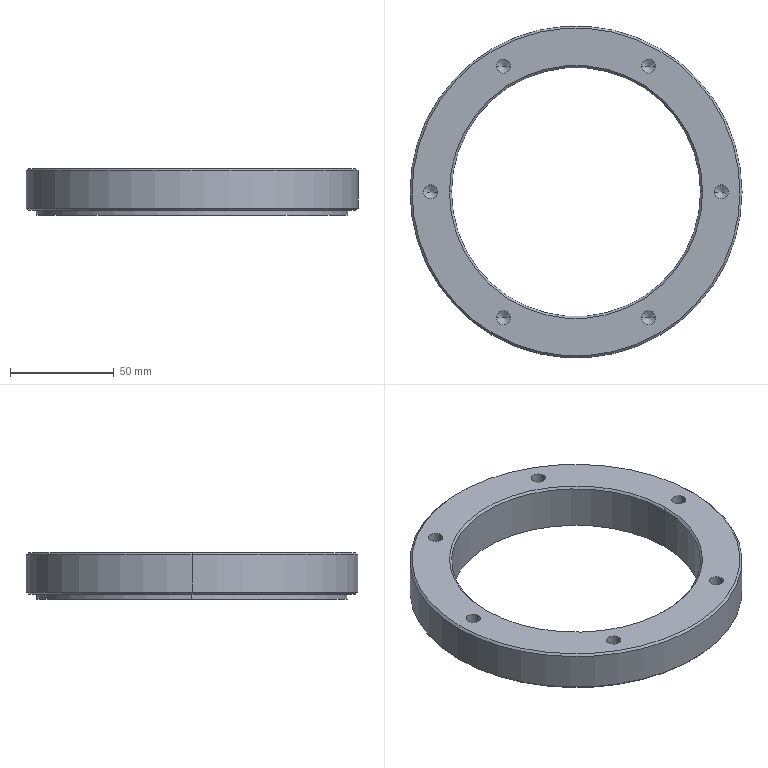Part | SolidWorks | features 3DProfileFeature 1, Chamfer 1, Extrusion 1, HoleWzd 1, ICE 1 | 1 solid | 45 faces | box 160 x 160 x 22.5 mm | volume 187073 mm3 | cylinder 18 | cone 18 | plane 9 | commonest cylinder face diameters 6.8 x12 120 x2 150 x2 160 x2
STEP:
#1=CARTESIAN_POINT('',(-75.,0.,-2.5));
#2=VERTEX_POINT('',#1);
#3=CARTESIAN_POINT('',(75.,0.,-2.5));
#4=VERTEX_POINT('',#3);
#5=CARTESIAN_POINT('',(0.,0.,-2.5));
#6=DIRECTION('',(0.,0.,-1.));
#7=DIRECTION('',(-1.,0.,0.));
#8=AXIS2_PLACEMENT_3D('',#5,#6,#7);
#9=CIRCLE('',#8,75.);
#10=EDGE_CURVE('',#2,#4,#9,.T.);
#11=ORIENTED_EDGE('',*,*,#10,.F.);
#12=CARTESIAN_POINT('',(-75.,0.,0.));
#13=VERTEX_POINT('',#12);
#14=CARTESIAN_POINT('',(-75.,0.,-2.5));
#15=DIRECTION('',(0.,0.,1.));
#16=VECTOR('',#15,1000.);
#17=LINE('',#14,#16);
#18=EDGE_CURVE('',#2,#13,#17,.T.);
#19=ORIENTED_EDGE('',*,*,#18,.T.);
#20=CARTESIAN_POINT('',(75.,0.,0.));
#21=VERTEX_POINT('',#20);
#22=CARTESIAN_POINT('',(0.,0.,0.));
#23=DIRECTION('',(0.,0.,-1.));
#24=DIRECTION('',(1.,0.,0.));
#25=AXIS2_PLACEMENT_3D('',#22,#23,#24);
#26=CIRCLE('',#25,75.);
#27=EDGE_CURVE('',#13,#21,#26,.T.);
#28=ORIENTED_EDGE('',*,*,#27,.T.);
#29=CARTESIAN_POINT('',(75.,0.,-2.5));
#30=DIRECTION('',(0.,0.,1.));
#31=VECTOR('',#30,1000.);
#32=LINE('',#29,#31);
#33=EDGE_CURVE('',#4,#21,#32,.T.);
#34=ORIENTED_EDGE('',*,*,#33,.F.);
#35=EDGE_LOOP('',(#11,#19,#28,#34));
#36=FACE_OUTER_BOUND('',#35,.T.);
#37=CARTESIAN_POINT('',(0.,0.,-2.5));
#38=DIRECTION('',(0.,0.,1.));
#39=DIRECTION('',(1.,0.,0.));
#40=AXIS2_PLACEMENT_3D('',#37,#38,#39);
#41=CYLINDRICAL_SURFACE('',#40,75.);
#42=ADVANCED_FACE('',(#36),#41,.T.);
#43=CARTESIAN_POINT('',(-60.,0.,19.));
#44=VERTEX_POINT('',#43);
#45=CARTESIAN_POINT('',(60.,0.,19.));
#46=VERTEX_POINT('',#45);
#47=CARTESIAN_POINT('',(0.,0.,19.));
#48=DIRECTION('',(0.,0.,1.));
#49=DIRECTION('',(1.,0.,0.));
#50=AXIS2_PLACEMENT_3D('',#47,#48,#49);
#51=CIRCLE('',#50,60.);
#52=EDGE_CURVE('',#44,#46,#51,.T.);
#53=ORIENTED_EDGE('',*,*,#52,.F.);
#54=CARTESIAN_POINT('',(-61.,0.,20.));
#55=VERTEX_POINT('',#54);
#56=CARTESIAN_POINT('',(-60.,0.,19.));
#57=DIRECTION('',(-0.7071,0.,0.7071));
#58=VECTOR('',#57,1000.);
#59=LINE('',#56,#58);
#60=EDGE_CURVE('',#44,#55,#59,.T.);
#61=ORIENTED_EDGE('',*,*,#60,.T.);
#62=CARTESIAN_POINT('',(61.,0.,20.));
#63=VERTEX_POINT('',#62);
#64=CARTESIAN_POINT('',(0.,0.,20.));
#65=DIRECTION('',(0.,0.,-1.));
#66=DIRECTION('',(1.,0.,0.));
#67=AXIS2_PLACEMENT_3D('',#64,#65,#66);
#68=CIRCLE('',#67,61.);
#69=EDGE_CURVE('',#63,#55,#68,.T.);
#70=ORIENTED_EDGE('',*,*,#69,.F.);
#71=CARTESIAN_POINT('',(60.,0.,19.));
#72=DIRECTION('',(0.7071,0.,0.7071));
#73=VECTOR('',#72,1000.);
#74=LINE('',#71,#73);
#75=EDGE_CURVE('',#46,#63,#74,.T.);
#76=ORIENTED_EDGE('',*,*,#75,.F.);
#77=EDGE_LOOP('',(#53,#61,#70,#76));
#78=FACE_OUTER_BOUND('',#77,.T.);
#79=CARTESIAN_POINT('',(0.,0.,19.));
#80=DIRECTION('',(0.,0.,1.));
#81=DIRECTION('',(1.,0.,0.));
#82=AXIS2_PLACEMENT_3D('',#79,#80,#81);
#83=CONICAL_SURFACE('',#82,60.,0.7854);
#84=ADVANCED_FACE('',(#78),#83,.F.);
#85=CARTESIAN_POINT('',(-79.,0.,0.));
#86=VERTEX_POINT('',#85);
#87=CARTESIAN_POINT('',(79.,0.,0.));
#88=VERTEX_POINT('',#87);
#89=CARTESIAN_POINT('',(0.,0.,0.));
#90=DIRECTION('',(0.,0.,-1.));
#91=DIRECTION('',(1.,0.,0.));
#92=AXIS2_PLACEMENT_3D('',#89,#90,#91);
#93=CIRCLE('',#92,79.);
#94=EDGE_CURVE('',#86,#88,#93,.T.);
#95=ORIENTED_EDGE('',*,*,#94,.F.);
#96=CARTESIAN_POINT('',(-80.,0.,1.));
#97=VERTEX_POINT('',#96);
#98=CARTESIAN_POINT('',(-80.,0.,1.));
#99=DIRECTION('',(-0.7071,0.,0.7071));
#100=VECTOR('',#99,1000.);
#101=LINE('',#98,#100);
#102=EDGE_CURVE('',#86,#97,#101,.T.);
#103=ORIENTED_EDGE('',*,*,#102,.T.);
#104=CARTESIAN_POINT('',(80.,0.,1.));
#105=VERTEX_POINT('',#104);
#106=CARTESIAN_POINT('',(0.,0.,1.));
#107=DIRECTION('',(0.,0.,1.));
#108=DIRECTION('',(1.,0.,0.));
#109=AXIS2_PLACEMENT_3D('',#106,#107,#108);
#110=CIRCLE('',#109,80.);
#111=EDGE_CURVE('',#105,#97,#110,.T.);
#112=ORIENTED_EDGE('',*,*,#111,.F.);
#113=CARTESIAN_POINT('',(80.,0.,1.));
#114=DIRECTION('',(0.7071,0.,0.7071));
#115=VECTOR('',#114,1000.);
#116=LINE('',#113,#115);
#117=EDGE_CURVE('',#88,#105,#116,.T.);
#118=ORIENTED_EDGE('',*,*,#117,.F.);
#119=EDGE_LOOP('',(#95,#103,#112,#118));
#120=FACE_OUTER_BOUND('',#119,.T.);
#121=CARTESIAN_POINT('',(0.,0.,1.));
#122=DIRECTION('',(0.,0.,1.));
#123=DIRECTION('',(1.,0.,0.));
#124=AXIS2_PLACEMENT_3D('',#121,#122,#123);
#125=CONICAL_SURFACE('',#124,80.,0.7854);
#126=ADVANCED_FACE('',(#120),#125,.T.);
#127=CARTESIAN_POINT('',(79.,0.,20.));
#128=VERTEX_POINT('',#127);
#129=CARTESIAN_POINT('',(-79.,0.,20.));
#130=VERTEX_POINT('',#129);
#131=CARTESIAN_POINT('',(0.,0.,20.));
#132=DIRECTION('',(0.,0.,1.));
#133=DIRECTION('',(1.,0.,0.));
#134=AXIS2_PLACEMENT_3D('',#131,#132,#133);
#135=CIRCLE('',#134,79.);
#136=EDGE_CURVE('',#128,#130,#135,.T.);
#137=ORIENTED_EDGE('',*,*,#136,.F.);
#138=CARTESIAN_POINT('',(80.,0.,19.));
#139=VERTEX_POINT('',#138);
#140=CARTESIAN_POINT('',(79.,0.,20.));
#141=DIRECTION('',(0.7071,0.,-0.7071));
#142=VECTOR('',#141,1000.);
#143=LINE('',#140,#142);
#144=EDGE_CURVE('',#128,#139,#143,.T.);
#145=ORIENTED_EDGE('',*,*,#144,.T.);
#146=CARTESIAN_POINT('',(-80.,0.,19.));
#147=VERTEX_POINT('',#146);
#148=CARTESIAN_POINT('',(0.,0.,19.));
#149=DIRECTION('',(0.,0.,-1.));
#150=DIRECTION('',(1.,0.,0.));
#151=AXIS2_PLACEMENT_3D('',#148,#149,#150);
#152=CIRCLE('',#151,80.);
#153=EDGE_CURVE('',#147,#139,#152,.T.);
#154=ORIENTED_EDGE('',*,*,#153,.F.);
#155=CARTESIAN_POINT('',(-79.,0.,20.));
#156=DIRECTION('',(-0.7071,0.,-0.7071));
#157=VECTOR('',#156,1000.);
#158=LINE('',#155,#157);
#159=EDGE_CURVE('',#130,#147,#158,.T.);
#160=ORIENTED_EDGE('',*,*,#159,.F.);
#161=EDGE_LOOP('',(#137,#145,#154,#160));
#162=FACE_OUTER_BOUND('',#161,.T.);
#163=CARTESIAN_POINT('',(0.,0.,20.));
#164=DIRECTION('',(0.,0.,-1.));
#165=DIRECTION('',(-1.,0.,0.));
#166=AXIS2_PLACEMENT_3D('',#163,#164,#165);
#167=CONICAL_SURFACE('',#166,79.,0.7854);
#168=ADVANCED_FACE('',(#162),#167,.T.);
#169=CARTESIAN_POINT('',(-38.4,60.622,2.));
#170=VERTEX_POINT('',#169);
#171=CARTESIAN_POINT('',(-31.6,60.622,2.));
#172=VERTEX_POINT('',#171);
#173=CARTESIAN_POINT('',(-35.,60.622,2.));
#174=DIRECTION('',(0.,0.,1.));
#175=DIRECTION('',(1.,0.,0.));
#176=AXIS2_PLACEMENT_3D('',#173,#174,#175);
#177=CIRCLE('',#176,3.4);
#178=EDGE_CURVE('',#170,#172,#177,.T.);
#179=ORIENTED_EDGE('',*,*,#178,.F.);
#180=CARTESIAN_POINT('',(-38.4,60.622,20.));
#181=VERTEX_POINT('',#180);
#182=CARTESIAN_POINT('',(-38.4,60.622,20.));
#183=DIRECTION('',(0.,0.,1.));
#184=VECTOR('',#183,1000.);
#185=LINE('',#182,#184);
#186=EDGE_CURVE('',#170,#181,#185,.T.);
#187=ORIENTED_EDGE('',*,*,#186,.T.);
#188=CARTESIAN_POINT('',(-31.6,60.622,20.));
#189=VERTEX_POINT('',#188);
#190=CARTESIAN_POINT('',(-35.,60.622,20.));
#191=DIRECTION('',(0.,0.,1.));
#192=DIRECTION('',(1.,0.,0.));
#193=AXIS2_PLACEMENT_3D('',#190,#191,#192);
#194=CIRCLE('',#193,3.4);
#195=EDGE_CURVE('',#181,#189,#194,.T.);
#196=ORIENTED_EDGE('',*,*,#195,.T.);
#197=CARTESIAN_POINT('',(-31.6,60.622,20.));
#198=DIRECTION('',(0.,0.,1.));
#199=VECTOR('',#198,1000.);
#200=LINE('',#197,#199);
#201=EDGE_CURVE('',#172,#189,#200,.T.);
#202=ORIENTED_EDGE('',*,*,#201,.F.);
#203=EDGE_LOOP('',(#179,#187,#196,#202));
#204=FACE_OUTER_BOUND('',#203,.T.);
#205=CARTESIAN_POINT('',(-35.,60.622,20.));
#206=DIRECTION('',(0.,0.,1.));
#207=DIRECTION('',(1.,0.,0.));
#208=AXIS2_PLACEMENT_3D('',#205,#206,#207);
#209=CYLINDRICAL_SURFACE('',#208,3.4);
#210=ADVANCED_FACE('',(#204),#209,.F.);
#211=CARTESIAN_POINT('',(-35.071,60.622,0.));
#212=VERTEX_POINT('',#211);
#213=CARTESIAN_POINT('',(-34.929,60.622,0.));
#214=VERTEX_POINT('',#213);
#215=CARTESIAN_POINT('',(-35.,60.622,0.));
#216=DIRECTION('',(0.,0.,1.));
#217=DIRECTION('',(1.,0.,0.));
#218=AXIS2_PLACEMENT_3D('',#215,#216,#217);
#219=CIRCLE('',#218,0.07144);
#220=EDGE_CURVE('',#212,#214,#219,.T.);
#221=ORIENTED_EDGE('',*,*,#220,.F.);
#222=CARTESIAN_POINT('',(-38.4,60.622,2.));
#223=DIRECTION('',(-0.8572,0.,0.515));
#224=VECTOR('',#223,1000.);
#225=LINE('',#222,#224);
#226=EDGE_CURVE('',#212,#170,#225,.T.);
#227=ORIENTED_EDGE('',*,*,#226,.T.);
#228=ORIENTED_EDGE('',*,*,#178,.T.);
#229=CARTESIAN_POINT('',(-31.6,60.622,2.));
#230=DIRECTION('',(0.8572,0.,0.515));
#231=VECTOR('',#230,1000.);
#232=LINE('',#229,#231);
#233=EDGE_CURVE('',#214,#172,#232,.T.);
#234=ORIENTED_EDGE('',*,*,#233,.F.);
#235=EDGE_LOOP('',(#221,#227,#228,#234));
#236=FACE_OUTER_BOUND('',#235,.T.);
#237=CARTESIAN_POINT('',(-35.,60.622,2.));
#238=DIRECTION('',(0.,0.,1.));
#239=DIRECTION('',(1.,0.,0.));
#240=AXIS2_PLACEMENT_3D('',#237,#238,#239);
#241=CONICAL_SURFACE('',#240,3.4,1.03);
#242=ADVANCED_FACE('',(#236),#241,.F.);
#243=CARTESIAN_POINT('',(-73.4,0.,2.));
#244=VERTEX_POINT('',#243);
#245=CARTESIAN_POINT('',(-66.6,0.,2.));
#246=VERTEX_POINT('',#245);
#247=CARTESIAN_POINT('',(-70.,0.,2.));
#248=DIRECTION('',(0.,0.,1.));
#249=DIRECTION('',(1.,0.,0.));
#250=AXIS2_PLACEMENT_3D('',#247,#248,#249);
#251=CIRCLE('',#250,3.4);
#252=EDGE_CURVE('',#244,#246,#251,.T.);
#253=ORIENTED_EDGE('',*,*,#252,.F.);
#254=CARTESIAN_POINT('',(-73.4,0.,20.));
#255=VERTEX_POINT('',#254);
#256=CARTESIAN_POINT('',(-73.4,0.,20.));
#257=DIRECTION('',(0.,0.,1.));
#258=VECTOR('',#257,1000.);
#259=LINE('',#256,#258);
#260=EDGE_CURVE('',#244,#255,#259,.T.);
#261=ORIENTED_EDGE('',*,*,#260,.T.);
#262=CARTESIAN_POINT('',(-66.6,0.,20.));
#263=VERTEX_POINT('',#262);
#264=CARTESIAN_POINT('',(-70.,0.,20.));
#265=DIRECTION('',(0.,0.,1.));
#266=DIRECTION('',(1.,0.,0.));
#267=AXIS2_PLACEMENT_3D('',#264,#265,#266);
#268=CIRCLE('',#267,3.4);
#269=EDGE_CURVE('',#255,#263,#268,.T.);
#270=ORIENTED_EDGE('',*,*,#269,.T.);
#271=CARTESIAN_POINT('',(-66.6,0.,20.));
#272=DIRECTION('',(0.,0.,1.));
#273=VECTOR('',#272,1000.);
#274=LINE('',#271,#273);
#275=EDGE_CURVE('',#246,#263,#274,.T.);
#276=ORIENTED_EDGE('',*,*,#275,.F.);
#277=EDGE_LOOP('',(#253,#261,#270,#276));
#278=FACE_OUTER_BOUND('',#277,.T.);
#279=CARTESIAN_POINT('',(-70.,0.,20.));
#280=DIRECTION('',(0.,0.,1.));
#281=DIRECTION('',(1.,0.,0.));
#282=AXIS2_PLACEMENT_3D('',#279,#280,#281);
#283=CYLINDRICAL_SURFACE('',#282,3.4);
#284=ADVANCED_FACE('',(#278),#283,.F.);
#285=CARTESIAN_POINT('',(-70.071,0.,0.));
#286=VERTEX_POINT('',#285);
#287=CARTESIAN_POINT('',(-69.929,0.,0.));
#288=VERTEX_POINT('',#287);
#289=CARTESIAN_POINT('',(-70.,0.,0.));
#290=DIRECTION('',(0.,0.,1.));
#291=DIRECTION('',(1.,0.,0.));
#292=AXIS2_PLACEMENT_3D('',#289,#290,#291);
#293=CIRCLE('',#292,0.07144);
#294=EDGE_CURVE('',#286,#288,#293,.T.);
#295=ORIENTED_EDGE('',*,*,#294,.F.);
#296=CARTESIAN_POINT('',(-73.4,0.,2.));
#297=DIRECTION('',(-0.8572,0.,0.515));
#298=VECTOR('',#297,1000.);
#299=LINE('',#296,#298);
#300=EDGE_CURVE('',#286,#244,#299,.T.);
#301=ORIENTED_EDGE('',*,*,#300,.T.);
#302=ORIENTED_EDGE('',*,*,#252,.T.);
#303=CARTESIAN_POINT('',(-66.6,0.,2.));
#304=DIRECTION('',(0.8572,0.,0.515));
#305=VECTOR('',#304,1000.);
#306=LINE('',#303,#305);
#307=EDGE_CURVE('',#288,#246,#306,.T.);
#308=ORIENTED_EDGE('',*,*,#307,.F.);
#309=EDGE_LOOP('',(#295,#301,#302,#308));
#310=FACE_OUTER_BOUND('',#309,.T.);
#311=CARTESIAN_POINT('',(-70.,0.,2.));
#312=DIRECTION('',(0.,0.,1.));
#313=DIRECTION('',(1.,0.,0.));
#314=AXIS2_PLACEMENT_3D('',#311,#312,#313);
#315=CONICAL_SURFACE('',#314,3.4,1.03);
#316=ADVANCED_FACE('',(#310),#315,.F.);
#317=CARTESIAN_POINT('',(-38.4,-60.622,2.));
#318=VERTEX_POINT('',#317);
#319=CARTESIAN_POINT('',(-31.6,-60.622,2.));
#320=VERTEX_POINT('',#319);
#321=CARTESIAN_POINT('',(-35.,-60.622,2.));
#322=DIRECTION('',(0.,0.,1.));
#323=DIRECTION('',(1.,0.,0.));
#324=AXIS2_PLACEMENT_3D('',#321,#322,#323);
#325=CIRCLE('',#324,3.4);
#326=EDGE_CURVE('',#318,#320,#325,.T.);
#327=ORIENTED_EDGE('',*,*,#326,.F.);
#328=CARTESIAN_POINT('',(-38.4,-60.622,20.));
#329=VERTEX_POINT('',#328);
#330=CARTESIAN_POINT('',(-38.4,-60.622,20.));
#331=DIRECTION('',(0.,0.,1.));
#332=VECTOR('',#331,1000.);
#333=LINE('',#330,#332);
#334=EDGE_CURVE('',#318,#329,#333,.T.);
#335=ORIENTED_EDGE('',*,*,#334,.T.);
#336=CARTESIAN_POINT('',(-31.6,-60.622,20.));
#337=VERTEX_POINT('',#336);
#338=CARTESIAN_POINT('',(-35.,-60.622,20.));
#339=DIRECTION('',(0.,0.,1.));
#340=DIRECTION('',(1.,0.,0.));
#341=AXIS2_PLACEMENT_3D('',#338,#339,#340);
#342=CIRCLE('',#341,3.4);
#343=EDGE_CURVE('',#329,#337,#342,.T.);
#344=ORIENTED_EDGE('',*,*,#343,.T.);
#345=CARTESIAN_POINT('',(-31.6,-60.622,20.));
#346=DIRECTION('',(0.,0.,1.));
#347=VECTOR('',#346,1000.);
#348=LINE('',#345,#347);
#349=EDGE_CURVE('',#320,#337,#348,.T.);
#350=ORIENTED_EDGE('',*,*,#349,.F.);
#351=EDGE_LOOP('',(#327,#335,#344,#350));
#352=FACE_OUTER_BOUND('',#351,.T.);
#353=CARTESIAN_POINT('',(-35.,-60.622,20.));
#354=DIRECTION('',(0.,0.,1.));
#355=DIRECTION('',(1.,0.,0.));
#356=AXIS2_PLACEMENT_3D('',#353,#354,#355);
#357=CYLINDRICAL_SURFACE('',#356,3.4);
#358=ADVANCED_FACE('',(#352),#357,.F.);
#359=CARTESIAN_POINT('',(-35.071,-60.622,0.));
#360=VERTEX_POINT('',#359);
#361=CARTESIAN_POINT('',(-34.929,-60.622,0.));
#362=VERTEX_POINT('',#361);
#363=CARTESIAN_POINT('',(-35.,-60.622,0.));
#364=DIRECTION('',(0.,0.,1.));
#365=DIRECTION('',(1.,0.,0.));
#366=AXIS2_PLACEMENT_3D('',#363,#364,#365);
#367=CIRCLE('',#366,0.07144);
#368=EDGE_CURVE('',#360,#362,#367,.T.);
#369=ORIENTED_EDGE('',*,*,#368,.F.);
#370=CARTESIAN_POINT('',(-38.4,-60.622,2.));
#371=DIRECTION('',(-0.8572,0.,0.515));
#372=VECTOR('',#371,1000.);
#373=LINE('',#370,#372);
#374=EDGE_CURVE('',#360,#318,#373,.T.);
#375=ORIENTED_EDGE('',*,*,#374,.T.);
#376=ORIENTED_EDGE('',*,*,#326,.T.);
#377=CARTESIAN_POINT('',(-31.6,-60.622,2.));
#378=DIRECTION('',(0.8572,0.,0.515));
#379=VECTOR('',#378,1000.);
#380=LINE('',#377,#379);
#381=EDGE_CURVE('',#362,#320,#380,.T.);
#382=ORIENTED_EDGE('',*,*,#381,.F.);
#383=EDGE_LOOP('',(#369,#375,#376,#382));
#384=FACE_OUTER_BOUND('',#383,.T.);
#385=CARTESIAN_POINT('',(-35.,-60.622,2.));
#386=DIRECTION('',(0.,0.,1.));
#387=DIRECTION('',(1.,0.,0.));
#388=AXIS2_PLACEMENT_3D('',#385,#386,#387);
#389=CONICAL_SURFACE('',#388,3.4,1.03);
#390=ADVANCED_FACE('',(#384),#389,.F.);
#391=CARTESIAN_POINT('',(31.6,-60.622,2.));
#392=VERTEX_POINT('',#391);
#393=CARTESIAN_POINT('',(38.4,-60.622,2.));
#394=VERTEX_POINT('',#393);
#395=CARTESIAN_POINT('',(35.,-60.622,2.));
#396=DIRECTION('',(0.,0.,1.));
#397=DIRECTION('',(1.,0.,0.));
#398=AXIS2_PLACEMENT_3D('',#395,#396,#397);
#399=CIRCLE('',#398,3.4);
#400=EDGE_CURVE('',#392,#394,#399,.T.);
#401=ORIENTED_EDGE('',*,*,#400,.F.);
#402=CARTESIAN_POINT('',(31.6,-60.622,20.));
#403=VERTEX_POINT('',#402);
#404=CARTESIAN_POINT('',(31.6,-60.622,20.));
#405=DIRECTION('',(0.,0.,1.));
#406=VECTOR('',#405,1000.);
#407=LINE('',#404,#406);
#408=EDGE_CURVE('',#392,#403,#407,.T.);
#409=ORIENTED_EDGE('',*,*,#408,.T.);
#410=CARTESIAN_POINT('',(38.4,-60.622,20.));
#411=VERTEX_POINT('',#410);
#412=CARTESIAN_POINT('',(35.,-60.622,20.));
#413=DIRECTION('',(0.,0.,1.));
#414=DIRECTION('',(1.,0.,0.));
#415=AXIS2_PLACEMENT_3D('',#412,#413,#414);
#416=CIRCLE('',#415,3.4);
#417=EDGE_CURVE('',#403,#411,#416,.T.);
#418=ORIENTED_EDGE('',*,*,#417,.T.);
#419=CARTESIAN_POINT('',(38.4,-60.622,20.));
#420=DIRECTION('',(0.,0.,1.));
#421=VECTOR('',#420,1000.);
#422=LINE('',#419,#421);
#423=EDGE_CURVE('',#394,#411,#422,.T.);
#424=ORIENTED_EDGE('',*,*,#423,.F.);
#425=EDGE_LOOP('',(#401,#409,#418,#424));
#426=FACE_OUTER_BOUND('',#425,.T.);
#427=CARTESIAN_POINT('',(35.,-60.622,20.));
#428=DIRECTION('',(0.,0.,1.));
#429=DIRECTION('',(1.,0.,0.));
#430=AXIS2_PLACEMENT_3D('',#427,#428,#429);
#431=CYLINDRICAL_SURFACE('',#430,3.4);
#432=ADVANCED_FACE('',(#426),#431,.F.);
#433=CARTESIAN_POINT('',(34.929,-60.622,0.));
#434=VERTEX_POINT('',#433);
#435=CARTESIAN_POINT('',(35.071,-60.622,0.));
#436=VERTEX_POINT('',#435);
#437=CARTESIAN_POINT('',(35.,-60.622,0.));
#438=DIRECTION('',(0.,0.,1.));
#439=DIRECTION('',(1.,0.,0.));
#440=AXIS2_PLACEMENT_3D('',#437,#438,#439);
#441=CIRCLE('',#440,0.07144);
#442=EDGE_CURVE('',#434,#436,#441,.T.);
#443=ORIENTED_EDGE('',*,*,#442,.F.);
#444=CARTESIAN_POINT('',(31.6,-60.622,2.));
#445=DIRECTION('',(-0.8572,0.,0.515));
#446=VECTOR('',#445,1000.);
#447=LINE('',#444,#446);
#448=EDGE_CURVE('',#434,#392,#447,.T.);
#449=ORIENTED_EDGE('',*,*,#448,.T.);
#450=ORIENTED_EDGE('',*,*,#400,.T.);
#451=CARTESIAN_POINT('',(38.4,-60.622,2.));
#452=DIRECTION('',(0.8572,0.,0.515));
#453=VECTOR('',#452,1000.);
#454=LINE('',#451,#453);
#455=EDGE_CURVE('',#436,#394,#454,.T.);
#456=ORIENTED_EDGE('',*,*,#455,.F.);
#457=EDGE_LOOP('',(#443,#449,#450,#456));
#458=FACE_OUTER_BOUND('',#457,.T.);
#459=CARTESIAN_POINT('',(35.,-60.622,2.));
#460=DIRECTION('',(0.,0.,1.));
#461=DIRECTION('',(1.,0.,0.));
#462=AXIS2_PLACEMENT_3D('',#459,#460,#461);
#463=CONICAL_SURFACE('',#462,3.4,1.03);
#464=ADVANCED_FACE('',(#458),#463,.F.);
#465=CARTESIAN_POINT('',(66.6,0.,2.));
#466=VERTEX_POINT('',#465);
#467=CARTESIAN_POINT('',(73.4,0.,2.));
#468=VERTEX_POINT('',#467);
#469=CARTESIAN_POINT('',(70.,0.,2.));
#470=DIRECTION('',(0.,0.,1.));
#471=DIRECTION('',(1.,0.,0.));
#472=AXIS2_PLACEMENT_3D('',#469,#470,#471);
#473=CIRCLE('',#472,3.4);
#474=EDGE_CURVE('',#466,#468,#473,.T.);
#475=ORIENTED_EDGE('',*,*,#474,.F.);
#476=CARTESIAN_POINT('',(66.6,0.,20.));
#477=VERTEX_POINT('',#476);
#478=CARTESIAN_POINT('',(66.6,0.,20.));
#479=DIRECTION('',(0.,0.,1.));
#480=VECTOR('',#479,1000.);
#481=LINE('',#478,#480);
#482=EDGE_CURVE('',#466,#477,#481,.T.);
#483=ORIENTED_EDGE('',*,*,#482,.T.);
#484=CARTESIAN_POINT('',(73.4,0.,20.));
#485=VERTEX_POINT('',#484);
#486=CARTESIAN_POINT('',(70.,0.,20.));
#487=DIRECTION('',(0.,0.,1.));
#488=DIRECTION('',(1.,0.,0.));
#489=AXIS2_PLACEMENT_3D('',#486,#487,#488);
#490=CIRCLE('',#489,3.4);
#491=EDGE_CURVE('',#477,#485,#490,.T.);
#492=ORIENTED_EDGE('',*,*,#491,.T.);
#493=CARTESIAN_POINT('',(73.4,0.,20.));
#494=DIRECTION('',(0.,0.,1.));
#495=VECTOR('',#494,1000.);
#496=LINE('',#493,#495);
#497=EDGE_CURVE('',#468,#485,#496,.T.);
#498=ORIENTED_EDGE('',*,*,#497,.F.);
#499=EDGE_LOOP('',(#475,#483,#492,#498));
#500=FACE_OUTER_BOUND('',#499,.T.);
#501=CARTESIAN_POINT('',(70.,0.,20.));
#502=DIRECTION('',(0.,0.,1.));
#503=DIRECTION('',(1.,0.,0.));
#504=AXIS2_PLACEMENT_3D('',#501,#502,#503);
#505=CYLINDRICAL_SURFACE('',#504,3.4);
#506=ADVANCED_FACE('',(#500),#505,.F.);
#507=CARTESIAN_POINT('',(69.929,0.,0.));
#508=VERTEX_POINT('',#507);
#509=CARTESIAN_POINT('',(70.071,0.,0.));
#510=VERTEX_POINT('',#509);
#511=CARTESIAN_POINT('',(70.,0.,0.));
#512=DIRECTION('',(0.,0.,1.));
#513=DIRECTION('',(1.,0.,0.));
#514=AXIS2_PLACEMENT_3D('',#511,#512,#513);
#515=CIRCLE('',#514,0.07144);
#516=EDGE_CURVE('',#508,#510,#515,.T.);
#517=ORIENTED_EDGE('',*,*,#516,.F.);
#518=CARTESIAN_POINT('',(66.6,0.,2.));
#519=DIRECTION('',(-0.8572,0.,0.515));
#520=VECTOR('',#519,1000.);
#521=LINE('',#518,#520);
#522=EDGE_CURVE('',#508,#466,#521,.T.);
#523=ORIENTED_EDGE('',*,*,#522,.T.);
#524=ORIENTED_EDGE('',*,*,#474,.T.);
#525=CARTESIAN_POINT('',(73.4,0.,2.));
#526=DIRECTION('',(0.8572,0.,0.515));
#527=VECTOR('',#526,1000.);
#528=LINE('',#525,#527);
#529=EDGE_CURVE('',#510,#468,#528,.T.);
#530=ORIENTED_EDGE('',*,*,#529,.F.);
#531=EDGE_LOOP('',(#517,#523,#524,#530));
#532=FACE_OUTER_BOUND('',#531,.T.);
#533=CARTESIAN_POINT('',(70.,0.,2.));
#534=DIRECTION('',(0.,0.,1.));
#535=DIRECTION('',(1.,0.,0.));
#536=AXIS2_PLACEMENT_3D('',#533,#534,#535);
#537=CONICAL_SURFACE('',#536,3.4,1.03);
#538=ADVANCED_FACE('',(#532),#537,.F.);
#539=CARTESIAN_POINT('',(31.6,60.622,2.));
#540=VERTEX_POINT('',#539);
#541=CARTESIAN_POINT('',(38.4,60.622,2.));
#542=VERTEX_POINT('',#541);
#543=CARTESIAN_POINT('',(35.,60.622,2.));
#544=DIRECTION('',(0.,0.,1.));
#545=DIRECTION('',(1.,0.,0.));
#546=AXIS2_PLACEMENT_3D('',#543,#544,#545);
#547=CIRCLE('',#546,3.4);
#548=EDGE_CURVE('',#540,#542,#547,.T.);
#549=ORIENTED_EDGE('',*,*,#548,.F.);
#550=CARTESIAN_POINT('',(31.6,60.622,20.));
#551=VERTEX_POINT('',#550);
#552=CARTESIAN_POINT('',(31.6,60.622,20.));
#553=DIRECTION('',(0.,0.,1.));
#554=VECTOR('',#553,1000.);
#555=LINE('',#552,#554);
#556=EDGE_CURVE('',#540,#551,#555,.T.);
#557=ORIENTED_EDGE('',*,*,#556,.T.);
#558=CARTESIAN_POINT('',(38.4,60.622,20.));
#559=VERTEX_POINT('',#558);
#560=CARTESIAN_POINT('',(35.,60.622,20.));
#561=DIRECTION('',(0.,0.,1.));
#562=DIRECTION('',(1.,0.,0.));
#563=AXIS2_PLACEMENT_3D('',#560,#561,#562);
#564=CIRCLE('',#563,3.4);
#565=EDGE_CURVE('',#551,#559,#564,.T.);
#566=ORIENTED_EDGE('',*,*,#565,.T.);
#567=CARTESIAN_POINT('',(38.4,60.622,20.));
#568=DIRECTION('',(0.,0.,1.));
#569=VECTOR('',#568,1000.);
#570=LINE('',#567,#569);
#571=EDGE_CURVE('',#542,#559,#570,.T.);
#572=ORIENTED_EDGE('',*,*,#571,.F.);
#573=EDGE_LOOP('',(#549,#557,#566,#572));
#574=FACE_OUTER_BOUND('',#573,.T.);
#575=CARTESIAN_POINT('',(35.,60.622,20.));
#576=DIRECTION('',(0.,0.,1.));
#577=DIRECTION('',(1.,0.,0.));
#578=AXIS2_PLACEMENT_3D('',#575,#576,#577);
#579=CYLINDRICAL_SURFACE('',#578,3.4);
#580=ADVANCED_FACE('',(#574),#579,.F.);
#581=CARTESIAN_POINT('',(34.929,60.622,0.));
#582=VERTEX_POINT('',#581);
#583=CARTESIAN_POINT('',(35.071,60.622,0.));
#584=VERTEX_POINT('',#583);
#585=CARTESIAN_POINT('',(35.,60.622,0.));
#586=DIRECTION('',(0.,0.,1.));
#587=DIRECTION('',(1.,0.,0.));
#588=AXIS2_PLACEMENT_3D('',#585,#586,#587);
#589=CIRCLE('',#588,0.07144);
#590=EDGE_CURVE('',#582,#584,#589,.T.);
#591=ORIENTED_EDGE('',*,*,#590,.F.);
#592=CARTESIAN_POINT('',(31.6,60.622,2.));
#593=DIRECTION('',(-0.8572,0.,0.515));
#594=VECTOR('',#593,1000.);
#595=LINE('',#592,#594);
#596=EDGE_CURVE('',#582,#540,#595,.T.);
#597=ORIENTED_EDGE('',*,*,#596,.T.);
#598=ORIENTED_EDGE('',*,*,#548,.T.);
#599=CARTESIAN_POINT('',(38.4,60.622,2.));
#600=DIRECTION('',(0.8572,0.,0.515));
#601=VECTOR('',#600,1000.);
#602=LINE('',#599,#601);
#603=EDGE_CURVE('',#584,#542,#602,.T.);
#604=ORIENTED_EDGE('',*,*,#603,.F.);
#605=EDGE_LOOP('',(#591,#597,#598,#604));
#606=FACE_OUTER_BOUND('',#605,.T.);
#607=CARTESIAN_POINT('',(35.,60.622,2.));
#608=DIRECTION('',(0.,0.,1.));
#609=DIRECTION('',(1.,0.,0.));
#610=AXIS2_PLACEMENT_3D('',#607,#608,#609);
#611=CONICAL_SURFACE('',#610,3.4,1.03);
#612=ADVANCED_FACE('',(#606),#611,.F.);
#613=ORIENTED_EDGE('',*,*,#52,.T.);
#614=CARTESIAN_POINT('',(60.,0.,-2.5));
#615=VERTEX_POINT('',#614);
#616=CARTESIAN_POINT('',(60.,0.,20.));
#617=DIRECTION('',(0.,0.,-1.));
#618=VECTOR('',#617,1000.);
#619=LINE('',#616,#618);
#620=EDGE_CURVE('',#46,#615,#619,.T.);
#621=ORIENTED_EDGE('',*,*,#620,.T.);
#622=CARTESIAN_POINT('',(-60.,0.,-2.5));
#623=VERTEX_POINT('',#622);
#624=CARTESIAN_POINT('',(0.,0.,-2.5));
#625=DIRECTION('',(0.,0.,-1.));
#626=DIRECTION('',(-1.,0.,0.));
#627=AXIS2_PLACEMENT_3D('',#624,#625,#626);
#628=CIRCLE('',#627,60.);
#629=EDGE_CURVE('',#615,#623,#628,.T.);
#630=ORIENTED_EDGE('',*,*,#629,.T.);
#631=CARTESIAN_POINT('',(-60.,0.,20.));
#632=DIRECTION('',(0.,0.,-1.));
#633=VECTOR('',#632,1000.);
#634=LINE('',#631,#633);
#635=EDGE_CURVE('',#44,#623,#634,.T.);
#636=ORIENTED_EDGE('',*,*,#635,.F.);
#637=EDGE_LOOP('',(#613,#621,#630,#636));
#638=FACE_OUTER_BOUND('',#637,.T.);
#639=CARTESIAN_POINT('',(0.,0.,20.));
#640=DIRECTION('',(0.,0.,-1.));
#641=DIRECTION('',(-1.,0.,0.));
#642=AXIS2_PLACEMENT_3D('',#639,#640,#641);
#643=CYLINDRICAL_SURFACE('',#642,60.);
#644=ADVANCED_FACE('',(#638),#643,.F.);
#645=ORIENTED_EDGE('',*,*,#153,.T.);
#646=CARTESIAN_POINT('',(80.,0.,20.));
#647=DIRECTION('',(0.,0.,-1.));
#648=VECTOR('',#647,1000.);
#649=LINE('',#646,#648);
#650=EDGE_CURVE('',#139,#105,#649,.T.);
#651=ORIENTED_EDGE('',*,*,#650,.T.);
#652=ORIENTED_EDGE('',*,*,#111,.T.);
#653=CARTESIAN_POINT('',(-80.,0.,20.));
#654=DIRECTION('',(0.,0.,-1.));
#655=VECTOR('',#654,1000.);
#656=LINE('',#653,#655);
#657=EDGE_CURVE('',#147,#97,#656,.T.);
#658=ORIENTED_EDGE('',*,*,#657,.F.);
#659=EDGE_LOOP('',(#645,#651,#652,#658));
#660=FACE_OUTER_BOUND('',#659,.T.);
#661=CARTESIAN_POINT('',(0.,0.,20.));
#662=DIRECTION('',(0.,0.,-1.));
#663=DIRECTION('',(-1.,0.,0.));
#664=AXIS2_PLACEMENT_3D('',#661,#662,#663);
#665=CYLINDRICAL_SURFACE('',#664,80.);
#666=ADVANCED_FACE('',(#660),#665,.T.);
#667=CARTESIAN_POINT('',(0.,0.,0.));
#668=DIRECTION('',(0.,0.,-1.));
#669=DIRECTION('',(1.,0.,0.));
#670=AXIS2_PLACEMENT_3D('',#667,#668,#669);
#671=CIRCLE('',#670,79.);
#672=EDGE_CURVE('',#88,#86,#671,.T.);
#673=ORIENTED_EDGE('',*,*,#672,.T.);
#674=ORIENTED_EDGE('',*,*,#94,.T.);
#675=EDGE_LOOP('',(#673,#674));
#676=FACE_OUTER_BOUND('',#675,.T.);
#677=CARTESIAN_POINT('',(0.,0.,0.));
#678=DIRECTION('',(0.,0.,-1.));
#679=DIRECTION('',(1.,0.,0.));
#680=AXIS2_PLACEMENT_3D('',#677,#678,#679);
#681=CIRCLE('',#680,75.);
#682=EDGE_CURVE('',#21,#13,#681,.T.);
#683=ORIENTED_EDGE('',*,*,#682,.F.);
#684=ORIENTED_EDGE('',*,*,#27,.F.);
#685=EDGE_LOOP('',(#683,#684));
#686=FACE_BOUND('',#685,.T.);
#687=CARTESIAN_POINT('',(0.,0.,0.));
#688=DIRECTION('',(0.,0.,1.));
#689=DIRECTION('',(1.,0.,0.));
#690=AXIS2_PLACEMENT_3D('',#687,#688,#689);
#691=PLANE('',#690);
#692=ADVANCED_FACE('',(#676,#686),#691,.F.);
#693=CARTESIAN_POINT('',(0.,0.,20.));
#694=DIRECTION('',(0.,0.,1.));
#695=DIRECTION('',(1.,0.,0.));
#696=AXIS2_PLACEMENT_3D('',#693,#694,#695);
#697=CIRCLE('',#696,79.);
#698=EDGE_CURVE('',#130,#128,#697,.T.);
#699=ORIENTED_EDGE('',*,*,#698,.T.);
#700=ORIENTED_EDGE('',*,*,#136,.T.);
#701=EDGE_LOOP('',(#699,#700));
#702=FACE_OUTER_BOUND('',#701,.T.);
#703=ORIENTED_EDGE('',*,*,#69,.T.);
#704=CARTESIAN_POINT('',(0.,0.,20.));
#705=DIRECTION('',(0.,0.,-1.));
#706=DIRECTION('',(1.,0.,0.));
#707=AXIS2_PLACEMENT_3D('',#704,#705,#706);
#708=CIRCLE('',#707,61.);
#709=EDGE_CURVE('',#55,#63,#708,.T.);
#710=ORIENTED_EDGE('',*,*,#709,.T.);
#711=EDGE_LOOP('',(#703,#710));
#712=FACE_BOUND('',#711,.T.);
#713=CARTESIAN_POINT('',(-35.,60.622,20.));
#714=DIRECTION('',(0.,0.,1.));
#715=DIRECTION('',(1.,0.,0.));
#716=AXIS2_PLACEMENT_3D('',#713,#714,#715);
#717=CIRCLE('',#716,3.4);
#718=EDGE_CURVE('',#189,#181,#717,.T.);
#719=ORIENTED_EDGE('',*,*,#718,.F.);
#720=ORIENTED_EDGE('',*,*,#195,.F.);
#721=EDGE_LOOP('',(#719,#720));
#722=FACE_BOUND('',#721,.T.);
#723=CARTESIAN_POINT('',(-70.,0.,20.));
#724=DIRECTION('',(0.,0.,1.));
#725=DIRECTION('',(1.,0.,0.));
#726=AXIS2_PLACEMENT_3D('',#723,#724,#725);
#727=CIRCLE('',#726,3.4);
#728=EDGE_CURVE('',#263,#255,#727,.T.);
#729=ORIENTED_EDGE('',*,*,#728,.F.);
#730=ORIENTED_EDGE('',*,*,#269,.F.);
#731=EDGE_LOOP('',(#729,#730));
#732=FACE_BOUND('',#731,.T.);
#733=CARTESIAN_POINT('',(-35.,-60.622,20.));
#734=DIRECTION('',(0.,0.,1.));
#735=DIRECTION('',(1.,0.,0.));
#736=AXIS2_PLACEMENT_3D('',#733,#734,#735);
#737=CIRCLE('',#736,3.4);
#738=EDGE_CURVE('',#337,#329,#737,.T.);
#739=ORIENTED_EDGE('',*,*,#738,.F.);
#740=ORIENTED_EDGE('',*,*,#343,.F.);
#741=EDGE_LOOP('',(#739,#740));
#742=FACE_BOUND('',#741,.T.);
#743=CARTESIAN_POINT('',(35.,-60.622,20.));
#744=DIRECTION('',(0.,0.,1.));
#745=DIRECTION('',(1.,0.,0.));
#746=AXIS2_PLACEMENT_3D('',#743,#744,#745);
#747=CIRCLE('',#746,3.4);
#748=EDGE_CURVE('',#411,#403,#747,.T.);
#749=ORIENTED_EDGE('',*,*,#748,.F.);
#750=ORIENTED_EDGE('',*,*,#417,.F.);
#751=EDGE_LOOP('',(#749,#750));
#752=FACE_BOUND('',#751,.T.);
#753=CARTESIAN_POINT('',(70.,0.,20.));
#754=DIRECTION('',(0.,0.,1.));
#755=DIRECTION('',(1.,0.,0.));
#756=AXIS2_PLACEMENT_3D('',#753,#754,#755);
#757=CIRCLE('',#756,3.4);
#758=EDGE_CURVE('',#485,#477,#757,.T.);
#759=ORIENTED_EDGE('',*,*,#758,.F.);
#760=ORIENTED_EDGE('',*,*,#491,.F.);
#761=EDGE_LOOP('',(#759,#760));
#762=FACE_BOUND('',#761,.T.);
#763=CARTESIAN_POINT('',(35.,60.622,20.));
#764=DIRECTION('',(0.,0.,1.));
#765=DIRECTION('',(1.,0.,0.));
#766=AXIS2_PLACEMENT_3D('',#763,#764,#765);
#767=CIRCLE('',#766,3.4);
#768=EDGE_CURVE('',#559,#551,#767,.T.);
#769=ORIENTED_EDGE('',*,*,#768,.F.);
#770=ORIENTED_EDGE('',*,*,#565,.F.);
#771=EDGE_LOOP('',(#769,#770));
#772=FACE_BOUND('',#771,.T.);
#773=CARTESIAN_POINT('',(0.,0.,20.));
#774=DIRECTION('',(0.,0.,1.));
#775=DIRECTION('',(1.,0.,0.));
#776=AXIS2_PLACEMENT_3D('',#773,#774,#775);
#777=PLANE('',#776);
#778=ADVANCED_FACE('',(#702,#712,#722,#732,#742,#752,#762,#772),#777,.T.);
#779=ORIENTED_EDGE('',*,*,#650,.F.);
#780=CARTESIAN_POINT('',(0.,0.,19.));
#781=DIRECTION('',(0.,0.,-1.));
#782=DIRECTION('',(1.,0.,0.));
#783=AXIS2_PLACEMENT_3D('',#780,#781,#782);
#784=CIRCLE('',#783,80.);
#785=EDGE_CURVE('',#139,#147,#784,.T.);
#786=ORIENTED_EDGE('',*,*,#785,.T.);
#787=ORIENTED_EDGE('',*,*,#657,.T.);
#788=CARTESIAN_POINT('',(0.,0.,1.));
#789=DIRECTION('',(0.,0.,1.));
#790=DIRECTION('',(1.,0.,0.));
#791=AXIS2_PLACEMENT_3D('',#788,#789,#790);
#792=CIRCLE('',#791,80.);
#793=EDGE_CURVE('',#97,#105,#792,.T.);
#794=ORIENTED_EDGE('',*,*,#793,.T.);
#795=EDGE_LOOP('',(#779,#786,#787,#794));
#796=FACE_OUTER_BOUND('',#795,.T.);
#797=CARTESIAN_POINT('',(0.,0.,20.));
#798=DIRECTION('',(0.,0.,-1.));
#799=DIRECTION('',(-1.,0.,0.));
#800=AXIS2_PLACEMENT_3D('',#797,#798,#799);
#801=CYLINDRICAL_SURFACE('',#800,80.);
#802=ADVANCED_FACE('',(#796),#801,.T.);
#803=ORIENTED_EDGE('',*,*,#620,.F.);
#804=CARTESIAN_POINT('',(0.,0.,19.));
#805=DIRECTION('',(0.,0.,1.));
#806=DIRECTION('',(1.,0.,0.));
#807=AXIS2_PLACEMENT_3D('',#804,#805,#806);
#808=CIRCLE('',#807,60.);
#809=EDGE_CURVE('',#46,#44,#808,.T.);
#810=ORIENTED_EDGE('',*,*,#809,.T.);
#811=ORIENTED_EDGE('',*,*,#635,.T.);
#812=CARTESIAN_POINT('',(0.,0.,-2.5));
#813=DIRECTION('',(0.,0.,-1.));
#814=DIRECTION('',(-1.,0.,0.));
#815=AXIS2_PLACEMENT_3D('',#812,#813,#814);
#816=CIRCLE('',#815,60.);
#817=EDGE_CURVE('',#623,#615,#816,.T.);
#818=ORIENTED_EDGE('',*,*,#817,.T.);
#819=EDGE_LOOP('',(#803,#810,#811,#818));
#820=FACE_OUTER_BOUND('',#819,.T.);
#821=CARTESIAN_POINT('',(0.,0.,20.));
#822=DIRECTION('',(0.,0.,-1.));
#823=DIRECTION('',(-1.,0.,0.));
#824=AXIS2_PLACEMENT_3D('',#821,#822,#823);
#825=CYLINDRICAL_SURFACE('',#824,60.);
#826=ADVANCED_FACE('',(#820),#825,.F.);
#827=ORIENTED_EDGE('',*,*,#596,.F.);
#828=CARTESIAN_POINT('',(35.,60.622,0.));
#829=DIRECTION('',(0.,0.,1.));
#830=DIRECTION('',(1.,0.,0.));
#831=AXIS2_PLACEMENT_3D('',#828,#829,#830);
#832=CIRCLE('',#831,0.07144);
#833=EDGE_CURVE('',#584,#582,#832,.T.);
#834=ORIENTED_EDGE('',*,*,#833,.F.);
#835=ORIENTED_EDGE('',*,*,#603,.T.);
#836=CARTESIAN_POINT('',(35.,60.622,2.));
#837=DIRECTION('',(0.,0.,1.));
#838=DIRECTION('',(1.,0.,0.));
#839=AXIS2_PLACEMENT_3D('',#836,#837,#838);
#840=CIRCLE('',#839,3.4);
#841=EDGE_CURVE('',#542,#540,#840,.T.);
#842=ORIENTED_EDGE('',*,*,#841,.T.);
#843=EDGE_LOOP('',(#827,#834,#835,#842));
#844=FACE_OUTER_BOUND('',#843,.T.);
#845=CARTESIAN_POINT('',(35.,60.622,2.));
#846=DIRECTION('',(0.,0.,1.));
#847=DIRECTION('',(1.,0.,0.));
#848=AXIS2_PLACEMENT_3D('',#845,#846,#847);
#849=CONICAL_SURFACE('',#848,3.4,1.03);
#850=ADVANCED_FACE('',(#844),#849,.F.);
#851=ORIENTED_EDGE('',*,*,#556,.F.);
#852=ORIENTED_EDGE('',*,*,#841,.F.);
#853=ORIENTED_EDGE('',*,*,#571,.T.);
#854=ORIENTED_EDGE('',*,*,#768,.T.);
#855=EDGE_LOOP('',(#851,#852,#853,#854));
#856=FACE_OUTER_BOUND('',#855,.T.);
#857=CARTESIAN_POINT('',(35.,60.622,20.));
#858=DIRECTION('',(0.,0.,1.));
#859=DIRECTION('',(1.,0.,0.));
#860=AXIS2_PLACEMENT_3D('',#857,#858,#859);
#861=CYLINDRICAL_SURFACE('',#860,3.4);
#862=ADVANCED_FACE('',(#856),#861,.F.);
#863=ORIENTED_EDGE('',*,*,#522,.F.);
#864=CARTESIAN_POINT('',(70.,0.,0.));
#865=DIRECTION('',(0.,0.,1.));
#866=DIRECTION('',(1.,0.,0.));
#867=AXIS2_PLACEMENT_3D('',#864,#865,#866);
#868=CIRCLE('',#867,0.07144);
#869=EDGE_CURVE('',#510,#508,#868,.T.);
#870=ORIENTED_EDGE('',*,*,#869,.F.);
#871=ORIENTED_EDGE('',*,*,#529,.T.);
#872=CARTESIAN_POINT('',(70.,0.,2.));
#873=DIRECTION('',(0.,0.,1.));
#874=DIRECTION('',(1.,0.,0.));
#875=AXIS2_PLACEMENT_3D('',#872,#873,#874);
#876=CIRCLE('',#875,3.4);
#877=EDGE_CURVE('',#468,#466,#876,.T.);
#878=ORIENTED_EDGE('',*,*,#877,.T.);
#879=EDGE_LOOP('',(#863,#870,#871,#878));
#880=FACE_OUTER_BOUND('',#879,.T.);
#881=CARTESIAN_POINT('',(70.,0.,2.));
#882=DIRECTION('',(0.,0.,1.));
#883=DIRECTION('',(1.,0.,0.));
#884=AXIS2_PLACEMENT_3D('',#881,#882,#883);
#885=CONICAL_SURFACE('',#884,3.4,1.03);
#886=ADVANCED_FACE('',(#880),#885,.F.);
#887=ORIENTED_EDGE('',*,*,#482,.F.);
#888=ORIENTED_EDGE('',*,*,#877,.F.);
#889=ORIENTED_EDGE('',*,*,#497,.T.);
#890=ORIENTED_EDGE('',*,*,#758,.T.);
#891=EDGE_LOOP('',(#887,#888,#889,#890));
#892=FACE_OUTER_BOUND('',#891,.T.);
#893=CARTESIAN_POINT('',(70.,0.,20.));
#894=DIRECTION('',(0.,0.,1.));
#895=DIRECTION('',(1.,0.,0.));
#896=AXIS2_PLACEMENT_3D('',#893,#894,#895);
#897=CYLINDRICAL_SURFACE('',#896,3.4);
#898=ADVANCED_FACE('',(#892),#897,.F.);
#899=ORIENTED_EDGE('',*,*,#448,.F.);
#900=CARTESIAN_POINT('',(35.,-60.622,0.));
#901=DIRECTION('',(0.,0.,1.));
#902=DIRECTION('',(1.,0.,0.));
#903=AXIS2_PLACEMENT_3D('',#900,#901,#902);
#904=CIRCLE('',#903,0.07144);
#905=EDGE_CURVE('',#436,#434,#904,.T.);
#906=ORIENTED_EDGE('',*,*,#905,.F.);
#907=ORIENTED_EDGE('',*,*,#455,.T.);
#908=CARTESIAN_POINT('',(35.,-60.622,2.));
#909=DIRECTION('',(0.,0.,1.));
#910=DIRECTION('',(1.,0.,0.));
#911=AXIS2_PLACEMENT_3D('',#908,#909,#910);
#912=CIRCLE('',#911,3.4);
#913=EDGE_CURVE('',#394,#392,#912,.T.);
#914=ORIENTED_EDGE('',*,*,#913,.T.);
#915=EDGE_LOOP('',(#899,#906,#907,#914));
#916=FACE_OUTER_BOUND('',#915,.T.);
#917=CARTESIAN_POINT('',(35.,-60.622,2.));
#918=DIRECTION('',(0.,0.,1.));
#919=DIRECTION('',(1.,0.,0.));
#920=AXIS2_PLACEMENT_3D('',#917,#918,#919);
#921=CONICAL_SURFACE('',#920,3.4,1.03);
#922=ADVANCED_FACE('',(#916),#921,.F.);
#923=ORIENTED_EDGE('',*,*,#408,.F.);
#924=ORIENTED_EDGE('',*,*,#913,.F.);
#925=ORIENTED_EDGE('',*,*,#423,.T.);
#926=ORIENTED_EDGE('',*,*,#748,.T.);
#927=EDGE_LOOP('',(#923,#924,#925,#926));
#928=FACE_OUTER_BOUND('',#927,.T.);
#929=CARTESIAN_POINT('',(35.,-60.622,20.));
#930=DIRECTION('',(0.,0.,1.));
#931=DIRECTION('',(1.,0.,0.));
#932=AXIS2_PLACEMENT_3D('',#929,#930,#931);
#933=CYLINDRICAL_SURFACE('',#932,3.4);
#934=ADVANCED_FACE('',(#928),#933,.F.);
#935=ORIENTED_EDGE('',*,*,#374,.F.);
#936=CARTESIAN_POINT('',(-35.,-60.622,0.));
#937=DIRECTION('',(0.,0.,1.));
#938=DIRECTION('',(1.,0.,0.));
#939=AXIS2_PLACEMENT_3D('',#936,#937,#938);
#940=CIRCLE('',#939,0.07144);
#941=EDGE_CURVE('',#362,#360,#940,.T.);
#942=ORIENTED_EDGE('',*,*,#941,.F.);
#943=ORIENTED_EDGE('',*,*,#381,.T.);
#944=CARTESIAN_POINT('',(-35.,-60.622,2.));
#945=DIRECTION('',(0.,0.,1.));
#946=DIRECTION('',(1.,0.,0.));
#947=AXIS2_PLACEMENT_3D('',#944,#945,#946);
#948=CIRCLE('',#947,3.4);
#949=EDGE_CURVE('',#320,#318,#948,.T.);
#950=ORIENTED_EDGE('',*,*,#949,.T.);
#951=EDGE_LOOP('',(#935,#942,#943,#950));
#952=FACE_OUTER_BOUND('',#951,.T.);
#953=CARTESIAN_POINT('',(-35.,-60.622,2.));
#954=DIRECTION('',(0.,0.,1.));
#955=DIRECTION('',(1.,0.,0.));
#956=AXIS2_PLACEMENT_3D('',#953,#954,#955);
#957=CONICAL_SURFACE('',#956,3.4,1.03);
#958=ADVANCED_FACE('',(#952),#957,.F.);
#959=ORIENTED_EDGE('',*,*,#334,.F.);
#960=ORIENTED_EDGE('',*,*,#949,.F.);
#961=ORIENTED_EDGE('',*,*,#349,.T.);
#962=ORIENTED_EDGE('',*,*,#738,.T.);
#963=EDGE_LOOP('',(#959,#960,#961,#962));
#964=FACE_OUTER_BOUND('',#963,.T.);
#965=CARTESIAN_POINT('',(-35.,-60.622,20.));
#966=DIRECTION('',(0.,0.,1.));
#967=DIRECTION('',(1.,0.,0.));
#968=AXIS2_PLACEMENT_3D('',#965,#966,#967);
#969=CYLINDRICAL_SURFACE('',#968,3.4);
#970=ADVANCED_FACE('',(#964),#969,.F.);
#971=ORIENTED_EDGE('',*,*,#300,.F.);
#972=CARTESIAN_POINT('',(-70.,0.,0.));
#973=DIRECTION('',(0.,0.,1.));
#974=DIRECTION('',(1.,0.,0.));
#975=AXIS2_PLACEMENT_3D('',#972,#973,#974);
#976=CIRCLE('',#975,0.07144);
#977=EDGE_CURVE('',#288,#286,#976,.T.);
#978=ORIENTED_EDGE('',*,*,#977,.F.);
#979=ORIENTED_EDGE('',*,*,#307,.T.);
#980=CARTESIAN_POINT('',(-70.,0.,2.));
#981=DIRECTION('',(0.,0.,1.));
#982=DIRECTION('',(1.,0.,0.));
#983=AXIS2_PLACEMENT_3D('',#980,#981,#982);
#984=CIRCLE('',#983,3.4);
#985=EDGE_CURVE('',#246,#244,#984,.T.);
#986=ORIENTED_EDGE('',*,*,#985,.T.);
#987=EDGE_LOOP('',(#971,#978,#979,#986));
#988=FACE_OUTER_BOUND('',#987,.T.);
#989=CARTESIAN_POINT('',(-70.,0.,2.));
#990=DIRECTION('',(0.,0.,1.));
#991=DIRECTION('',(1.,0.,0.));
#992=AXIS2_PLACEMENT_3D('',#989,#990,#991);
#993=CONICAL_SURFACE('',#992,3.4,1.03);
#994=ADVANCED_FACE('',(#988),#993,.F.);
#995=ORIENTED_EDGE('',*,*,#260,.F.);
#996=ORIENTED_EDGE('',*,*,#985,.F.);
#997=ORIENTED_EDGE('',*,*,#275,.T.);
#998=ORIENTED_EDGE('',*,*,#728,.T.);
#999=EDGE_LOOP('',(#995,#996,#997,#998));
#1000=FACE_OUTER_BOUND('',#999,.T.);
#1001=CARTESIAN_POINT('',(-70.,0.,20.));
#1002=DIRECTION('',(0.,0.,1.));
#1003=DIRECTION('',(1.,0.,0.));
#1004=AXIS2_PLACEMENT_3D('',#1001,#1002,#1003);
#1005=CYLINDRICAL_SURFACE('',#1004,3.4);
#1006=ADVANCED_FACE('',(#1000),#1005,.F.);
#1007=ORIENTED_EDGE('',*,*,#226,.F.);
#1008=CARTESIAN_POINT('',(-35.,60.622,0.));
#1009=DIRECTION('',(0.,0.,1.));
#1010=DIRECTION('',(1.,0.,0.));
#1011=AXIS2_PLACEMENT_3D('',#1008,#1009,#1010);
#1012=CIRCLE('',#1011,0.07144);
#1013=EDGE_CURVE('',#214,#212,#1012,.T.);
#1014=ORIENTED_EDGE('',*,*,#1013,.F.);
#1015=ORIENTED_EDGE('',*,*,#233,.T.);
#1016=CARTESIAN_POINT('',(-35.,60.622,2.));
#1017=DIRECTION('',(0.,0.,1.));
#1018=DIRECTION('',(1.,0.,0.));
#1019=AXIS2_PLACEMENT_3D('',#1016,#1017,#1018);
#1020=CIRCLE('',#1019,3.4);
#1021=EDGE_CURVE('',#172,#170,#1020,.T.);
#1022=ORIENTED_EDGE('',*,*,#1021,.T.);
#1023=EDGE_LOOP('',(#1007,#1014,#1015,#1022));
#1024=FACE_OUTER_BOUND('',#1023,.T.);
#1025=CARTESIAN_POINT('',(-35.,60.622,2.));
#1026=DIRECTION('',(0.,0.,1.));
#1027=DIRECTION('',(1.,0.,0.));
#1028=AXIS2_PLACEMENT_3D('',#1025,#1026,#1027);
#1029=CONICAL_SURFACE('',#1028,3.4,1.03);
#1030=ADVANCED_FACE('',(#1024),#1029,.F.);
#1031=ORIENTED_EDGE('',*,*,#186,.F.);
#1032=ORIENTED_EDGE('',*,*,#1021,.F.);
#1033=ORIENTED_EDGE('',*,*,#201,.T.);
#1034=ORIENTED_EDGE('',*,*,#718,.T.);
#1035=EDGE_LOOP('',(#1031,#1032,#1033,#1034));
#1036=FACE_OUTER_BOUND('',#1035,.T.);
#1037=CARTESIAN_POINT('',(-35.,60.622,20.));
#1038=DIRECTION('',(0.,0.,1.));
#1039=DIRECTION('',(1.,0.,0.));
#1040=AXIS2_PLACEMENT_3D('',#1037,#1038,#1039);
#1041=CYLINDRICAL_SURFACE('',#1040,3.4);
#1042=ADVANCED_FACE('',(#1036),#1041,.F.);
#1043=ORIENTED_EDGE('',*,*,#144,.F.);
#1044=ORIENTED_EDGE('',*,*,#698,.F.);
#1045=ORIENTED_EDGE('',*,*,#159,.T.);
#1046=ORIENTED_EDGE('',*,*,#785,.F.);
#1047=EDGE_LOOP('',(#1043,#1044,#1045,#1046));
#1048=FACE_OUTER_BOUND('',#1047,.T.);
#1049=CARTESIAN_POINT('',(0.,0.,20.));
#1050=DIRECTION('',(0.,0.,-1.));
#1051=DIRECTION('',(-1.,0.,0.));
#1052=AXIS2_PLACEMENT_3D('',#1049,#1050,#1051);
#1053=CONICAL_SURFACE('',#1052,79.,0.7854);
#1054=ADVANCED_FACE('',(#1048),#1053,.T.);
#1055=ORIENTED_EDGE('',*,*,#102,.F.);
#1056=ORIENTED_EDGE('',*,*,#672,.F.);
#1057=ORIENTED_EDGE('',*,*,#117,.T.);
#1058=ORIENTED_EDGE('',*,*,#793,.F.);
#1059=EDGE_LOOP('',(#1055,#1056,#1057,#1058));
#1060=FACE_OUTER_BOUND('',#1059,.T.);
#1061=CARTESIAN_POINT('',(0.,0.,1.));
#1062=DIRECTION('',(0.,0.,1.));
#1063=DIRECTION('',(1.,0.,0.));
#1064=AXIS2_PLACEMENT_3D('',#1061,#1062,#1063);
#1065=CONICAL_SURFACE('',#1064,80.,0.7854);
#1066=ADVANCED_FACE('',(#1060),#1065,.T.);
#1067=ORIENTED_EDGE('',*,*,#60,.F.);
#1068=ORIENTED_EDGE('',*,*,#809,.F.);
#1069=ORIENTED_EDGE('',*,*,#75,.T.);
#1070=ORIENTED_EDGE('',*,*,#709,.F.);
#1071=EDGE_LOOP('',(#1067,#1068,#1069,#1070));
#1072=FACE_OUTER_BOUND('',#1071,.T.);
#1073=CARTESIAN_POINT('',(0.,0.,19.));
#1074=DIRECTION('',(0.,0.,1.));
#1075=DIRECTION('',(1.,0.,0.));
#1076=AXIS2_PLACEMENT_3D('',#1073,#1074,#1075);
#1077=CONICAL_SURFACE('',#1076,60.,0.7854);
#1078=ADVANCED_FACE('',(#1072),#1077,.F.);
#1079=ORIENTED_EDGE('',*,*,#1013,.T.);
#1080=ORIENTED_EDGE('',*,*,#220,.T.);
#1081=EDGE_LOOP('',(#1079,#1080));
#1082=FACE_OUTER_BOUND('',#1081,.T.);
#1083=CARTESIAN_POINT('',(0.,0.,0.));
#1084=DIRECTION('',(0.,0.,-1.));
#1085=DIRECTION('',(-1.,0.,0.));
#1086=AXIS2_PLACEMENT_3D('',#1083,#1084,#1085);
#1087=PLANE('',#1086);
#1088=ADVANCED_FACE('',(#1082),#1087,.F.);
#1089=ORIENTED_EDGE('',*,*,#977,.T.);
#1090=ORIENTED_EDGE('',*,*,#294,.T.);
#1091=EDGE_LOOP('',(#1089,#1090));
#1092=FACE_OUTER_BOUND('',#1091,.T.);
#1093=CARTESIAN_POINT('',(0.,0.,0.));
#1094=DIRECTION('',(0.,0.,-1.));
#1095=DIRECTION('',(-1.,0.,0.));
#1096=AXIS2_PLACEMENT_3D('',#1093,#1094,#1095);
#1097=PLANE('',#1096);
#1098=ADVANCED_FACE('',(#1092),#1097,.F.);
#1099=ORIENTED_EDGE('',*,*,#941,.T.);
#1100=ORIENTED_EDGE('',*,*,#368,.T.);
#1101=EDGE_LOOP('',(#1099,#1100));
#1102=FACE_OUTER_BOUND('',#1101,.T.);
#1103=CARTESIAN_POINT('',(0.,0.,0.));
#1104=DIRECTION('',(0.,0.,-1.));
#1105=DIRECTION('',(-1.,0.,0.));
#1106=AXIS2_PLACEMENT_3D('',#1103,#1104,#1105);
#1107=PLANE('',#1106);
#1108=ADVANCED_FACE('',(#1102),#1107,.F.);
#1109=ORIENTED_EDGE('',*,*,#905,.T.);
#1110=ORIENTED_EDGE('',*,*,#442,.T.);
#1111=EDGE_LOOP('',(#1109,#1110));
#1112=FACE_OUTER_BOUND('',#1111,.T.);
#1113=CARTESIAN_POINT('',(0.,0.,0.));
#1114=DIRECTION('',(0.,0.,-1.));
#1115=DIRECTION('',(-1.,0.,0.));
#1116=AXIS2_PLACEMENT_3D('',#1113,#1114,#1115);
#1117=PLANE('',#1116);
#1118=ADVANCED_FACE('',(#1112),#1117,.F.);
#1119=ORIENTED_EDGE('',*,*,#869,.T.);
#1120=ORIENTED_EDGE('',*,*,#516,.T.);
#1121=EDGE_LOOP('',(#1119,#1120));
#1122=FACE_OUTER_BOUND('',#1121,.T.);
#1123=CARTESIAN_POINT('',(0.,0.,0.));
#1124=DIRECTION('',(0.,0.,-1.));
#1125=DIRECTION('',(-1.,0.,0.));
#1126=AXIS2_PLACEMENT_3D('',#1123,#1124,#1125);
#1127=PLANE('',#1126);
#1128=ADVANCED_FACE('',(#1122),#1127,.F.);
#1129=ORIENTED_EDGE('',*,*,#833,.T.);
#1130=ORIENTED_EDGE('',*,*,#590,.T.);
#1131=EDGE_LOOP('',(#1129,#1130));
#1132=FACE_OUTER_BOUND('',#1131,.T.);
#1133=CARTESIAN_POINT('',(0.,0.,0.));
#1134=DIRECTION('',(0.,0.,-1.));
#1135=DIRECTION('',(-1.,0.,0.));
#1136=AXIS2_PLACEMENT_3D('',#1133,#1134,#1135);
#1137=PLANE('',#1136);
#1138=ADVANCED_FACE('',(#1132),#1137,.F.);
#1139=CARTESIAN_POINT('',(0.,0.,-2.5));
#1140=DIRECTION('',(0.,0.,-1.));
#1141=DIRECTION('',(-1.,0.,0.));
#1142=AXIS2_PLACEMENT_3D('',#1139,#1140,#1141);
#1143=CIRCLE('',#1142,75.);
#1144=EDGE_CURVE('',#4,#2,#1143,.T.);
#1145=ORIENTED_EDGE('',*,*,#1144,.T.);
#1146=ORIENTED_EDGE('',*,*,#10,.T.);
#1147=EDGE_LOOP('',(#1145,#1146));
#1148=FACE_OUTER_BOUND('',#1147,.T.);
#1149=ORIENTED_EDGE('',*,*,#817,.F.);
#1150=ORIENTED_EDGE('',*,*,#629,.F.);
#1151=EDGE_LOOP('',(#1149,#1150));
#1152=FACE_BOUND('',#1151,.T.);
#1153=CARTESIAN_POINT('',(0.,0.,-2.5));
#1154=DIRECTION('',(0.,0.,-1.));
#1155=DIRECTION('',(-1.,0.,0.));
#1156=AXIS2_PLACEMENT_3D('',#1153,#1154,#1155);
#1157=PLANE('',#1156);
#1158=ADVANCED_FACE('',(#1148,#1152),#1157,.T.);
#1159=ORIENTED_EDGE('',*,*,#18,.F.);
#1160=ORIENTED_EDGE('',*,*,#1144,.F.);
#1161=ORIENTED_EDGE('',*,*,#33,.T.);
#1162=ORIENTED_EDGE('',*,*,#682,.T.);
#1163=EDGE_LOOP('',(#1159,#1160,#1161,#1162));
#1164=FACE_OUTER_BOUND('',#1163,.T.);
#1165=CARTESIAN_POINT('',(0.,0.,-2.5));
#1166=DIRECTION('',(0.,0.,1.));
#1167=DIRECTION('',(1.,0.,0.));
#1168=AXIS2_PLACEMENT_3D('',#1165,#1166,#1167);
#1169=CYLINDRICAL_SURFACE('',#1168,75.);
#1170=ADVANCED_FACE('',(#1164),#1169,.T.);
#1171=CLOSED_SHELL('',(#42,#84,#126,#168,#210,#242,#284,#316,#358,#390,#432,#464,#506,#538,#580,#612,#644,#666,#692,#778,#802,#826,#850,#862,#886,#898,#922,#934,#958,#970,#994,#1006,#1030,#1042,#1054,#1066,#1078,#1088,#1098,#1108,#1118,#1128,#1138,#1158,#1170));
#1172=MANIFOLD_SOLID_BREP('',#1171);
#1173=CARTESIAN_POINT('',(0.,0.,0.));
#1174=DIRECTION('',(0.,0.,1.));
#1175=DIRECTION('',(1.,0.,0.));
#1176=AXIS2_PLACEMENT_3D('',#1173,#1174,#1175);
#1177=(LENGTH_UNIT()NAMED_UNIT(*)SI_UNIT(.MILLI.,.METRE.));
#1178=UNCERTAINTY_MEASURE_WITH_UNIT(LENGTH_MEASURE(0.00001),#1177,'','');
#1179=(NAMED_UNIT(*)PLANE_ANGLE_UNIT()SI_UNIT($,.RADIAN.));
#1180=(NAMED_UNIT(*)SI_UNIT($,.STERADIAN.)SOLID_ANGLE_UNIT());
#1181=(GEOMETRIC_REPRESENTATION_CONTEXT(3)GLOBAL_UNCERTAINTY_ASSIGNED_CONTEXT((#1178))GLOBAL_UNIT_ASSIGNED_CONTEXT((#1177,#1179,#1180))REPRESENTATION_CONTEXT('',''));
#1182=ADVANCED_BREP_SHAPE_REPRESENTATION('',(#1172,#1176),#1181);